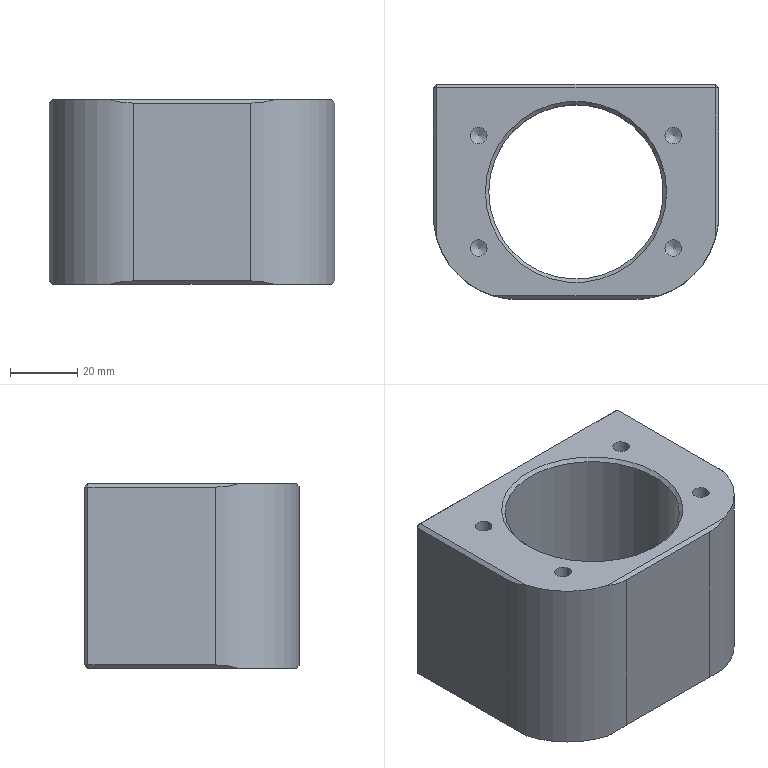Part | NX | 1 solid | 49 faces | box 85 x 64 x 55 mm | volume 163326 mm3 | plane 20 | cylinder 15 | cone 14 | commonest cylinder face diameters 2.5 x4 5 x4 6.8 x4 50 x2 52 x1
STEP:
#1=CARTESIAN_POINT('',(42.5,31.,54.));
#2=VERTEX_POINT('',#1);
#3=CARTESIAN_POINT('',(42.5,-7.,54.));
#4=VERTEX_POINT('',#3);
#5=CARTESIAN_POINT('',(42.5,-32.,54.));
#6=DIRECTION('',(0.,-1.,0.));
#7=VECTOR('',#6,1000.);
#8=LINE('',#5,#7);
#9=EDGE_CURVE('',#2,#4,#8,.T.);
#10=ORIENTED_EDGE('',*,*,#9,.T.);
#11=CARTESIAN_POINT('',(42.5,-7.,1.));
#12=VERTEX_POINT('',#11);
#13=CARTESIAN_POINT('',(42.5,-7.,55.));
#14=DIRECTION('',(0.,0.,-1.));
#15=VECTOR('',#14,1000.);
#16=LINE('',#13,#15);
#17=EDGE_CURVE('',#4,#12,#16,.T.);
#18=ORIENTED_EDGE('',*,*,#17,.T.);
#19=CARTESIAN_POINT('',(42.5,31.,1.));
#20=VERTEX_POINT('',#19);
#21=CARTESIAN_POINT('',(42.5,32.,1.));
#22=DIRECTION('',(0.,1.,0.));
#23=VECTOR('',#22,1000.);
#24=LINE('',#21,#23);
#25=EDGE_CURVE('',#12,#20,#24,.T.);
#26=ORIENTED_EDGE('',*,*,#25,.T.);
#27=CARTESIAN_POINT('',(42.5,31.,55.));
#28=DIRECTION('',(0.,0.,1.));
#29=VECTOR('',#28,1000.);
#30=LINE('',#27,#29);
#31=EDGE_CURVE('',#20,#2,#30,.T.);
#32=ORIENTED_EDGE('',*,*,#31,.T.);
#33=EDGE_LOOP('',(#10,#18,#26,#32));
#34=FACE_BOUND('',#33,.T.);
#35=CARTESIAN_POINT('',(42.5,-32.,55.));
#36=DIRECTION('',(-1.,0.,0.));
#37=DIRECTION('',(0.,0.,1.));
#38=AXIS2_PLACEMENT_3D('',#35,#36,#37);
#39=PLANE('',#38);
#40=ADVANCED_FACE('',(#34),#39,.F.);
#41=CARTESIAN_POINT('',(41.5,32.,54.));
#42=VERTEX_POINT('',#41);
#43=CARTESIAN_POINT('',(41.5,32.,1.));
#44=VERTEX_POINT('',#43);
#45=CARTESIAN_POINT('',(41.5,32.,55.));
#46=DIRECTION('',(0.,0.,-1.));
#47=VECTOR('',#46,1000.);
#48=LINE('',#45,#47);
#49=EDGE_CURVE('',#42,#44,#48,.T.);
#50=ORIENTED_EDGE('',*,*,#49,.T.);
#51=CARTESIAN_POINT('',(-41.5,32.,1.));
#52=VERTEX_POINT('',#51);
#53=CARTESIAN_POINT('',(-42.5,32.,1.));
#54=DIRECTION('',(-1.,0.,0.));
#55=VECTOR('',#54,1000.);
#56=LINE('',#53,#55);
#57=EDGE_CURVE('',#44,#52,#56,.T.);
#58=ORIENTED_EDGE('',*,*,#57,.T.);
#59=CARTESIAN_POINT('',(-41.5,32.,54.));
#60=VERTEX_POINT('',#59);
#61=CARTESIAN_POINT('',(-41.5,32.,55.));
#62=DIRECTION('',(0.,0.,1.));
#63=VECTOR('',#62,1000.);
#64=LINE('',#61,#63);
#65=EDGE_CURVE('',#52,#60,#64,.T.);
#66=ORIENTED_EDGE('',*,*,#65,.T.);
#67=CARTESIAN_POINT('',(-42.5,32.,54.));
#68=DIRECTION('',(1.,0.,0.));
#69=VECTOR('',#68,1000.);
#70=LINE('',#67,#69);
#71=EDGE_CURVE('',#60,#42,#70,.T.);
#72=ORIENTED_EDGE('',*,*,#71,.T.);
#73=EDGE_LOOP('',(#50,#58,#66,#72));
#74=FACE_BOUND('',#73,.T.);
#75=CARTESIAN_POINT('',(35.,32.,13.4));
#76=VERTEX_POINT('',#75);
#77=CARTESIAN_POINT('',(35.,32.,10.));
#78=DIRECTION('',(0.,1.,0.));
#79=DIRECTION('',(0.,0.,1.));
#80=AXIS2_PLACEMENT_3D('',#77,#78,#79);
#81=CIRCLE('',#80,3.4);
#82=EDGE_CURVE('',#76,#76,#81,.T.);
#83=ORIENTED_EDGE('',*,*,#82,.F.);
#84=EDGE_LOOP('',(#83));
#85=FACE_BOUND('',#84,.T.);
#86=CARTESIAN_POINT('',(-35.,32.,13.4));
#87=VERTEX_POINT('',#86);
#88=CARTESIAN_POINT('',(-35.,32.,10.));
#89=DIRECTION('',(0.,1.,0.));
#90=DIRECTION('',(0.,0.,1.));
#91=AXIS2_PLACEMENT_3D('',#88,#89,#90);
#92=CIRCLE('',#91,3.4);
#93=EDGE_CURVE('',#87,#87,#92,.T.);
#94=ORIENTED_EDGE('',*,*,#93,.F.);
#95=EDGE_LOOP('',(#94));
#96=FACE_BOUND('',#95,.T.);
#97=CARTESIAN_POINT('',(35.,32.,48.4));
#98=VERTEX_POINT('',#97);
#99=CARTESIAN_POINT('',(35.,32.,45.));
#100=DIRECTION('',(0.,1.,0.));
#101=DIRECTION('',(0.,0.,1.));
#102=AXIS2_PLACEMENT_3D('',#99,#100,#101);
#103=CIRCLE('',#102,3.4);
#104=EDGE_CURVE('',#98,#98,#103,.T.);
#105=ORIENTED_EDGE('',*,*,#104,.F.);
#106=EDGE_LOOP('',(#105));
#107=FACE_BOUND('',#106,.T.);
#108=CARTESIAN_POINT('',(-35.,32.,48.4));
#109=VERTEX_POINT('',#108);
#110=CARTESIAN_POINT('',(-35.,32.,45.));
#111=DIRECTION('',(0.,1.,0.));
#112=DIRECTION('',(0.,0.,1.));
#113=AXIS2_PLACEMENT_3D('',#110,#111,#112);
#114=CIRCLE('',#113,3.4);
#115=EDGE_CURVE('',#109,#109,#114,.T.);
#116=ORIENTED_EDGE('',*,*,#115,.F.);
#117=EDGE_LOOP('',(#116));
#118=FACE_BOUND('',#117,.T.);
#119=CARTESIAN_POINT('',(-42.5,32.,55.));
#120=DIRECTION('',(0.,-1.,0.));
#121=DIRECTION('',(0.,0.,-1.));
#122=AXIS2_PLACEMENT_3D('',#119,#120,#121);
#123=PLANE('',#122);
#124=ADVANCED_FACE('',(#74,#85,#96,#107,#118),#123,.F.);
#125=CARTESIAN_POINT('',(-42.5,31.,1.));
#126=VERTEX_POINT('',#125);
#127=CARTESIAN_POINT('',(-42.5,-7.,1.));
#128=VERTEX_POINT('',#127);
#129=CARTESIAN_POINT('',(-42.5,-32.,1.));
#130=DIRECTION('',(0.,-1.,0.));
#131=VECTOR('',#130,1000.);
#132=LINE('',#129,#131);
#133=EDGE_CURVE('',#126,#128,#132,.T.);
#134=ORIENTED_EDGE('',*,*,#133,.T.);
#135=CARTESIAN_POINT('',(-42.5,-7.,54.));
#136=VERTEX_POINT('',#135);
#137=CARTESIAN_POINT('',(-42.5,-7.,55.));
#138=DIRECTION('',(0.,0.,-1.));
#139=VECTOR('',#138,1000.);
#140=LINE('',#137,#139);
#141=EDGE_CURVE('',#128,#136,#140,.F.);
#142=ORIENTED_EDGE('',*,*,#141,.T.);
#143=CARTESIAN_POINT('',(-42.5,31.,54.));
#144=VERTEX_POINT('',#143);
#145=CARTESIAN_POINT('',(-42.5,-32.,54.));
#146=DIRECTION('',(0.,1.,0.));
#147=VECTOR('',#146,1000.);
#148=LINE('',#145,#147);
#149=EDGE_CURVE('',#136,#144,#148,.T.);
#150=ORIENTED_EDGE('',*,*,#149,.T.);
#151=CARTESIAN_POINT('',(-42.5,31.,55.));
#152=DIRECTION('',(0.,0.,-1.));
#153=VECTOR('',#152,1000.);
#154=LINE('',#151,#153);
#155=EDGE_CURVE('',#144,#126,#154,.T.);
#156=ORIENTED_EDGE('',*,*,#155,.T.);
#157=EDGE_LOOP('',(#134,#142,#150,#156));
#158=FACE_BOUND('',#157,.T.);
#159=CARTESIAN_POINT('',(-42.5,-32.,55.));
#160=DIRECTION('',(1.,0.,0.));
#161=DIRECTION('',(0.,0.,-1.));
#162=AXIS2_PLACEMENT_3D('',#159,#160,#161);
#163=PLANE('',#162);
#164=ADVANCED_FACE('',(#158),#163,.F.);
#165=CARTESIAN_POINT('',(17.5,-32.,54.));
#166=VERTEX_POINT('',#165);
#167=CARTESIAN_POINT('',(-17.5,-32.,54.));
#168=VERTEX_POINT('',#167);
#169=CARTESIAN_POINT('',(-42.5,-32.,54.));
#170=DIRECTION('',(-1.,0.,0.));
#171=VECTOR('',#170,1000.);
#172=LINE('',#169,#171);
#173=EDGE_CURVE('',#166,#168,#172,.T.);
#174=ORIENTED_EDGE('',*,*,#173,.T.);
#175=CARTESIAN_POINT('',(-17.5,-32.,1.));
#176=VERTEX_POINT('',#175);
#177=CARTESIAN_POINT('',(-17.5,-32.,55.));
#178=DIRECTION('',(0.,0.,-1.));
#179=VECTOR('',#178,1000.);
#180=LINE('',#177,#179);
#181=EDGE_CURVE('',#168,#176,#180,.T.);
#182=ORIENTED_EDGE('',*,*,#181,.T.);
#183=CARTESIAN_POINT('',(17.5,-32.,1.));
#184=VERTEX_POINT('',#183);
#185=CARTESIAN_POINT('',(42.5,-32.,1.));
#186=DIRECTION('',(1.,0.,0.));
#187=VECTOR('',#186,1000.);
#188=LINE('',#185,#187);
#189=EDGE_CURVE('',#176,#184,#188,.T.);
#190=ORIENTED_EDGE('',*,*,#189,.T.);
#191=CARTESIAN_POINT('',(17.5,-32.,55.));
#192=DIRECTION('',(0.,0.,-1.));
#193=VECTOR('',#192,1000.);
#194=LINE('',#191,#193);
#195=EDGE_CURVE('',#184,#166,#194,.F.);
#196=ORIENTED_EDGE('',*,*,#195,.T.);
#197=EDGE_LOOP('',(#174,#182,#190,#196));
#198=FACE_BOUND('',#197,.T.);
#199=CARTESIAN_POINT('',(-42.5,-32.,55.));
#200=DIRECTION('',(0.,1.,0.));
#201=DIRECTION('',(0.,0.,1.));
#202=AXIS2_PLACEMENT_3D('',#199,#200,#201);
#203=PLANE('',#202);
#204=ADVANCED_FACE('',(#198),#203,.F.);
#205=CARTESIAN_POINT('',(-27.,0.,55.));
#206=VERTEX_POINT('',#205);
#207=CARTESIAN_POINT('',(0.,0.,55.));
#208=DIRECTION('',(0.,0.,-1.));
#209=DIRECTION('',(-1.,0.,0.));
#210=AXIS2_PLACEMENT_3D('',#207,#208,#209);
#211=CIRCLE('',#210,27.);
#212=EDGE_CURVE('',#206,#206,#211,.T.);
#213=ORIENTED_EDGE('',*,*,#212,.T.);
#214=EDGE_LOOP('',(#213));
#215=FACE_BOUND('',#214,.T.);
#216=CARTESIAN_POINT('',(-41.5,31.,55.));
#217=VERTEX_POINT('',#216);
#218=CARTESIAN_POINT('',(-41.5,-14.,55.));
#219=VERTEX_POINT('',#218);
#220=CARTESIAN_POINT('',(-41.5,32.,55.));
#221=DIRECTION('',(0.,-1.,0.));
#222=VECTOR('',#221,1000.);
#223=LINE('',#220,#222);
#224=EDGE_CURVE('',#217,#219,#223,.T.);
#225=ORIENTED_EDGE('',*,*,#224,.T.);
#226=CARTESIAN_POINT('',(-24.5,-31.,55.));
#227=VERTEX_POINT('',#226);
#228=CARTESIAN_POINT('',(-17.5,-7.,55.));
#229=DIRECTION('',(0.,0.,-1.));
#230=DIRECTION('',(-1.,0.,0.));
#231=AXIS2_PLACEMENT_3D('',#228,#229,#230);
#232=CIRCLE('',#231,25.);
#233=EDGE_CURVE('',#219,#227,#232,.F.);
#234=ORIENTED_EDGE('',*,*,#233,.T.);
#235=CARTESIAN_POINT('',(24.5,-31.,55.));
#236=VERTEX_POINT('',#235);
#237=CARTESIAN_POINT('',(42.5,-31.,55.));
#238=DIRECTION('',(1.,0.,0.));
#239=VECTOR('',#238,1000.);
#240=LINE('',#237,#239);
#241=EDGE_CURVE('',#227,#236,#240,.T.);
#242=ORIENTED_EDGE('',*,*,#241,.T.);
#243=CARTESIAN_POINT('',(41.5,-14.,55.));
#244=VERTEX_POINT('',#243);
#245=CARTESIAN_POINT('',(17.5,-7.,55.));
#246=DIRECTION('',(0.,0.,-1.));
#247=DIRECTION('',(-1.,0.,0.));
#248=AXIS2_PLACEMENT_3D('',#245,#246,#247);
#249=CIRCLE('',#248,25.);
#250=EDGE_CURVE('',#236,#244,#249,.F.);
#251=ORIENTED_EDGE('',*,*,#250,.T.);
#252=CARTESIAN_POINT('',(41.5,31.,55.));
#253=VERTEX_POINT('',#252);
#254=CARTESIAN_POINT('',(41.5,32.,55.));
#255=DIRECTION('',(0.,1.,0.));
#256=VECTOR('',#255,1000.);
#257=LINE('',#254,#256);
#258=EDGE_CURVE('',#244,#253,#257,.T.);
#259=ORIENTED_EDGE('',*,*,#258,.T.);
#260=CARTESIAN_POINT('',(42.5,31.,55.));
#261=DIRECTION('',(-1.,0.,0.));
#262=VECTOR('',#261,1000.);
#263=LINE('',#260,#262);
#264=EDGE_CURVE('',#253,#217,#263,.T.);
#265=ORIENTED_EDGE('',*,*,#264,.T.);
#266=EDGE_LOOP('',(#225,#234,#242,#251,#259,#265));
#267=FACE_BOUND('',#266,.T.);
#268=CARTESIAN_POINT('',(31.512,16.75,55.));
#269=VERTEX_POINT('',#268);
#270=CARTESIAN_POINT('',(29.012,16.75,55.));
#271=DIRECTION('',(0.,0.,1.));
#272=DIRECTION('',(1.,0.,0.));
#273=AXIS2_PLACEMENT_3D('',#270,#271,#272);
#274=CIRCLE('',#273,2.5);
#275=EDGE_CURVE('',#269,#269,#274,.T.);
#276=ORIENTED_EDGE('',*,*,#275,.F.);
#277=EDGE_LOOP('',(#276));
#278=FACE_BOUND('',#277,.T.);
#279=CARTESIAN_POINT('',(-26.512,16.75,55.));
#280=VERTEX_POINT('',#279);
#281=CARTESIAN_POINT('',(-29.012,16.75,55.));
#282=DIRECTION('',(0.,0.,1.));
#283=DIRECTION('',(1.,0.,0.));
#284=AXIS2_PLACEMENT_3D('',#281,#282,#283);
#285=CIRCLE('',#284,2.5);
#286=EDGE_CURVE('',#280,#280,#285,.T.);
#287=ORIENTED_EDGE('',*,*,#286,.F.);
#288=EDGE_LOOP('',(#287));
#289=FACE_BOUND('',#288,.T.);
#290=CARTESIAN_POINT('',(-26.512,-16.75,55.));
#291=VERTEX_POINT('',#290);
#292=CARTESIAN_POINT('',(-29.012,-16.75,55.));
#293=DIRECTION('',(0.,0.,1.));
#294=DIRECTION('',(1.,0.,0.));
#295=AXIS2_PLACEMENT_3D('',#292,#293,#294);
#296=CIRCLE('',#295,2.5);
#297=EDGE_CURVE('',#291,#291,#296,.T.);
#298=ORIENTED_EDGE('',*,*,#297,.F.);
#299=EDGE_LOOP('',(#298));
#300=FACE_BOUND('',#299,.T.);
#301=CARTESIAN_POINT('',(31.512,-16.75,55.));
#302=VERTEX_POINT('',#301);
#303=CARTESIAN_POINT('',(29.012,-16.75,55.));
#304=DIRECTION('',(0.,0.,1.));
#305=DIRECTION('',(1.,0.,0.));
#306=AXIS2_PLACEMENT_3D('',#303,#304,#305);
#307=CIRCLE('',#306,2.5);
#308=EDGE_CURVE('',#302,#302,#307,.T.);
#309=ORIENTED_EDGE('',*,*,#308,.F.);
#310=EDGE_LOOP('',(#309));
#311=FACE_BOUND('',#310,.T.);
#312=CARTESIAN_POINT('',(42.5,32.,55.));
#313=DIRECTION('',(0.,0.,-1.));
#314=DIRECTION('',(-1.,0.,0.));
#315=AXIS2_PLACEMENT_3D('',#312,#313,#314);
#316=PLANE('',#315);
#317=ADVANCED_FACE('',(#215,#267,#278,#289,#300,#311),#316,.F.);
#318=CARTESIAN_POINT('',(28.75,22.,0.));
#319=VERTEX_POINT('',#318);
#320=CARTESIAN_POINT('',(30.,22.,0.));
#321=DIRECTION('',(0.,0.,-1.));
#322=DIRECTION('',(-1.,0.,0.));
#323=AXIS2_PLACEMENT_3D('',#320,#321,#322);
#324=CIRCLE('',#323,1.25);
#325=EDGE_CURVE('',#319,#319,#324,.T.);
#326=ORIENTED_EDGE('',*,*,#325,.F.);
#327=EDGE_LOOP('',(#326));
#328=FACE_BOUND('',#327,.T.);
#329=CARTESIAN_POINT('',(-31.25,22.,0.));
#330=VERTEX_POINT('',#329);
#331=CARTESIAN_POINT('',(-30.,22.,0.));
#332=DIRECTION('',(0.,0.,-1.));
#333=DIRECTION('',(-1.,0.,0.));
#334=AXIS2_PLACEMENT_3D('',#331,#332,#333);
#335=CIRCLE('',#334,1.25);
#336=EDGE_CURVE('',#330,#330,#335,.T.);
#337=ORIENTED_EDGE('',*,*,#336,.F.);
#338=EDGE_LOOP('',(#337));
#339=FACE_BOUND('',#338,.T.);
#340=CARTESIAN_POINT('',(-31.25,-13.,0.));
#341=VERTEX_POINT('',#340);
#342=CARTESIAN_POINT('',(-30.,-13.,0.));
#343=DIRECTION('',(0.,0.,-1.));
#344=DIRECTION('',(-1.,0.,0.));
#345=AXIS2_PLACEMENT_3D('',#342,#343,#344);
#346=CIRCLE('',#345,1.25);
#347=EDGE_CURVE('',#341,#341,#346,.T.);
#348=ORIENTED_EDGE('',*,*,#347,.F.);
#349=EDGE_LOOP('',(#348));
#350=FACE_BOUND('',#349,.T.);
#351=CARTESIAN_POINT('',(28.75,-13.,0.));
#352=VERTEX_POINT('',#351);
#353=CARTESIAN_POINT('',(30.,-13.,0.));
#354=DIRECTION('',(0.,0.,-1.));
#355=DIRECTION('',(-1.,0.,0.));
#356=AXIS2_PLACEMENT_3D('',#353,#354,#355);
#357=CIRCLE('',#356,1.25);
#358=EDGE_CURVE('',#352,#352,#357,.T.);
#359=ORIENTED_EDGE('',*,*,#358,.F.);
#360=EDGE_LOOP('',(#359));
#361=FACE_BOUND('',#360,.T.);
#362=CARTESIAN_POINT('',(-27.,0.,0.));
#363=VERTEX_POINT('',#362);
#364=CARTESIAN_POINT('',(0.,0.,0.));
#365=DIRECTION('',(0.,0.,-1.));
#366=DIRECTION('',(-1.,0.,0.));
#367=AXIS2_PLACEMENT_3D('',#364,#365,#366);
#368=CIRCLE('',#367,27.);
#369=EDGE_CURVE('',#363,#363,#368,.F.);
#370=ORIENTED_EDGE('',*,*,#369,.T.);
#371=EDGE_LOOP('',(#370));
#372=FACE_BOUND('',#371,.T.);
#373=CARTESIAN_POINT('',(24.5,-31.,0.));
#374=VERTEX_POINT('',#373);
#375=CARTESIAN_POINT('',(-24.5,-31.,0.));
#376=VERTEX_POINT('',#375);
#377=CARTESIAN_POINT('',(-42.5,-31.,0.));
#378=DIRECTION('',(-1.,0.,0.));
#379=VECTOR('',#378,1000.);
#380=LINE('',#377,#379);
#381=EDGE_CURVE('',#374,#376,#380,.T.);
#382=ORIENTED_EDGE('',*,*,#381,.T.);
#383=CARTESIAN_POINT('',(-41.5,-14.,0.));
#384=VERTEX_POINT('',#383);
#385=CARTESIAN_POINT('',(-17.5,-7.,0.));
#386=DIRECTION('',(0.,0.,-1.));
#387=DIRECTION('',(-1.,0.,0.));
#388=AXIS2_PLACEMENT_3D('',#385,#386,#387);
#389=CIRCLE('',#388,25.);
#390=EDGE_CURVE('',#376,#384,#389,.T.);
#391=ORIENTED_EDGE('',*,*,#390,.T.);
#392=CARTESIAN_POINT('',(-41.5,31.,0.));
#393=VERTEX_POINT('',#392);
#394=CARTESIAN_POINT('',(-41.5,32.,0.));
#395=DIRECTION('',(0.,1.,0.));
#396=VECTOR('',#395,1000.);
#397=LINE('',#394,#396);
#398=EDGE_CURVE('',#384,#393,#397,.T.);
#399=ORIENTED_EDGE('',*,*,#398,.T.);
#400=CARTESIAN_POINT('',(41.5,31.,0.));
#401=VERTEX_POINT('',#400);
#402=CARTESIAN_POINT('',(42.5,31.,0.));
#403=DIRECTION('',(1.,0.,0.));
#404=VECTOR('',#403,1000.);
#405=LINE('',#402,#404);
#406=EDGE_CURVE('',#393,#401,#405,.T.);
#407=ORIENTED_EDGE('',*,*,#406,.T.);
#408=CARTESIAN_POINT('',(41.5,-14.,0.));
#409=VERTEX_POINT('',#408);
#410=CARTESIAN_POINT('',(41.5,-32.,0.));
#411=DIRECTION('',(0.,-1.,0.));
#412=VECTOR('',#411,1000.);
#413=LINE('',#410,#412);
#414=EDGE_CURVE('',#401,#409,#413,.T.);
#415=ORIENTED_EDGE('',*,*,#414,.T.);
#416=CARTESIAN_POINT('',(17.5,-7.,0.));
#417=DIRECTION('',(0.,0.,-1.));
#418=DIRECTION('',(-1.,0.,0.));
#419=AXIS2_PLACEMENT_3D('',#416,#417,#418);
#420=CIRCLE('',#419,25.);
#421=EDGE_CURVE('',#409,#374,#420,.T.);
#422=ORIENTED_EDGE('',*,*,#421,.T.);
#423=EDGE_LOOP('',(#382,#391,#399,#407,#415,#422));
#424=FACE_BOUND('',#423,.T.);
#425=CARTESIAN_POINT('',(42.5,32.,0.));
#426=DIRECTION('',(0.,0.,-1.));
#427=DIRECTION('',(-1.,0.,0.));
#428=AXIS2_PLACEMENT_3D('',#425,#426,#427);
#429=PLANE('',#428);
#430=ADVANCED_FACE('',(#328,#339,#350,#361,#372,#424),#429,.T.);
#431=CARTESIAN_POINT('',(-26.,0.,54.));
#432=VERTEX_POINT('',#431);
#433=CARTESIAN_POINT('',(0.,0.,54.));
#434=DIRECTION('',(0.,0.,-1.));
#435=DIRECTION('',(-1.,0.,0.));
#436=AXIS2_PLACEMENT_3D('',#433,#434,#435);
#437=CIRCLE('',#436,26.);
#438=EDGE_CURVE('',#432,#432,#437,.F.);
#439=ORIENTED_EDGE('',*,*,#438,.T.);
#440=EDGE_LOOP('',(#439));
#441=FACE_BOUND('',#440,.T.);
#442=CARTESIAN_POINT('',(-26.,0.,1.));
#443=VERTEX_POINT('',#442);
#444=CARTESIAN_POINT('',(0.,0.,1.));
#445=DIRECTION('',(0.,0.,-1.));
#446=DIRECTION('',(-1.,0.,0.));
#447=AXIS2_PLACEMENT_3D('',#444,#445,#446);
#448=CIRCLE('',#447,26.);
#449=EDGE_CURVE('',#443,#443,#448,.T.);
#450=ORIENTED_EDGE('',*,*,#449,.T.);
#451=EDGE_LOOP('',(#450));
#452=FACE_BOUND('',#451,.T.);
#453=CARTESIAN_POINT('',(0.,0.,0.));
#454=DIRECTION('',(0.,0.,1.));
#455=DIRECTION('',(1.,0.,0.));
#456=AXIS2_PLACEMENT_3D('',#453,#454,#455);
#457=CYLINDRICAL_SURFACE('',#456,26.);
#458=ADVANCED_FACE('',(#441,#452),#457,.F.);
#459=CARTESIAN_POINT('',(-35.,13.457,45.));
#460=VERTEX_POINT('',#459);
#461=VERTEX_LOOP('',#460);
#462=FACE_BOUND('',#461,.T.);
#463=CARTESIAN_POINT('',(-35.,15.5,48.4));
#464=VERTEX_POINT('',#463);
#465=CARTESIAN_POINT('',(-35.,15.5,45.));
#466=DIRECTION('',(0.,1.,0.));
#467=DIRECTION('',(0.,0.,1.));
#468=AXIS2_PLACEMENT_3D('',#465,#466,#467);
#469=CIRCLE('',#468,3.4);
#470=EDGE_CURVE('',#464,#464,#469,.T.);
#471=ORIENTED_EDGE('',*,*,#470,.T.);
#472=EDGE_LOOP('',(#471));
#473=FACE_BOUND('',#472,.T.);
#474=CARTESIAN_POINT('',(-35.,15.5,45.));
#475=DIRECTION('',(0.,1.,0.));
#476=DIRECTION('',(0.,0.,1.));
#477=AXIS2_PLACEMENT_3D('',#474,#475,#476);
#478=CONICAL_SURFACE('',#477,3.4,1.03);
#479=ADVANCED_FACE('',(#462,#473),#478,.F.);
#480=ORIENTED_EDGE('',*,*,#470,.F.);
#481=EDGE_LOOP('',(#480));
#482=FACE_BOUND('',#481,.T.);
#483=ORIENTED_EDGE('',*,*,#115,.T.);
#484=EDGE_LOOP('',(#483));
#485=FACE_BOUND('',#484,.T.);
#486=CARTESIAN_POINT('',(-35.,32.,45.));
#487=DIRECTION('',(0.,1.,0.));
#488=DIRECTION('',(0.,0.,1.));
#489=AXIS2_PLACEMENT_3D('',#486,#487,#488);
#490=CYLINDRICAL_SURFACE('',#489,3.4);
#491=ADVANCED_FACE('',(#482,#485),#490,.F.);
#492=CARTESIAN_POINT('',(35.,13.457,45.));
#493=VERTEX_POINT('',#492);
#494=VERTEX_LOOP('',#493);
#495=FACE_BOUND('',#494,.T.);
#496=CARTESIAN_POINT('',(35.,15.5,48.4));
#497=VERTEX_POINT('',#496);
#498=CARTESIAN_POINT('',(35.,15.5,45.));
#499=DIRECTION('',(0.,1.,0.));
#500=DIRECTION('',(0.,0.,1.));
#501=AXIS2_PLACEMENT_3D('',#498,#499,#500);
#502=CIRCLE('',#501,3.4);
#503=EDGE_CURVE('',#497,#497,#502,.T.);
#504=ORIENTED_EDGE('',*,*,#503,.T.);
#505=EDGE_LOOP('',(#504));
#506=FACE_BOUND('',#505,.T.);
#507=CARTESIAN_POINT('',(35.,15.5,45.));
#508=DIRECTION('',(0.,1.,0.));
#509=DIRECTION('',(0.,0.,1.));
#510=AXIS2_PLACEMENT_3D('',#507,#508,#509);
#511=CONICAL_SURFACE('',#510,3.4,1.03);
#512=ADVANCED_FACE('',(#495,#506),#511,.F.);
#513=ORIENTED_EDGE('',*,*,#503,.F.);
#514=EDGE_LOOP('',(#513));
#515=FACE_BOUND('',#514,.T.);
#516=ORIENTED_EDGE('',*,*,#104,.T.);
#517=EDGE_LOOP('',(#516));
#518=FACE_BOUND('',#517,.T.);
#519=CARTESIAN_POINT('',(35.,32.,45.));
#520=DIRECTION('',(0.,1.,0.));
#521=DIRECTION('',(0.,0.,1.));
#522=AXIS2_PLACEMENT_3D('',#519,#520,#521);
#523=CYLINDRICAL_SURFACE('',#522,3.4);
#524=ADVANCED_FACE('',(#515,#518),#523,.F.);
#525=CARTESIAN_POINT('',(-35.,13.457,10.));
#526=VERTEX_POINT('',#525);
#527=VERTEX_LOOP('',#526);
#528=FACE_BOUND('',#527,.T.);
#529=CARTESIAN_POINT('',(-35.,15.5,13.4));
#530=VERTEX_POINT('',#529);
#531=CARTESIAN_POINT('',(-35.,15.5,10.));
#532=DIRECTION('',(0.,1.,0.));
#533=DIRECTION('',(0.,0.,1.));
#534=AXIS2_PLACEMENT_3D('',#531,#532,#533);
#535=CIRCLE('',#534,3.4);
#536=EDGE_CURVE('',#530,#530,#535,.T.);
#537=ORIENTED_EDGE('',*,*,#536,.T.);
#538=EDGE_LOOP('',(#537));
#539=FACE_BOUND('',#538,.T.);
#540=CARTESIAN_POINT('',(-35.,15.5,10.));
#541=DIRECTION('',(0.,1.,0.));
#542=DIRECTION('',(0.,0.,1.));
#543=AXIS2_PLACEMENT_3D('',#540,#541,#542);
#544=CONICAL_SURFACE('',#543,3.4,1.03);
#545=ADVANCED_FACE('',(#528,#539),#544,.F.);
#546=ORIENTED_EDGE('',*,*,#536,.F.);
#547=EDGE_LOOP('',(#546));
#548=FACE_BOUND('',#547,.T.);
#549=ORIENTED_EDGE('',*,*,#93,.T.);
#550=EDGE_LOOP('',(#549));
#551=FACE_BOUND('',#550,.T.);
#552=CARTESIAN_POINT('',(-35.,32.,10.));
#553=DIRECTION('',(0.,1.,0.));
#554=DIRECTION('',(0.,0.,1.));
#555=AXIS2_PLACEMENT_3D('',#552,#553,#554);
#556=CYLINDRICAL_SURFACE('',#555,3.4);
#557=ADVANCED_FACE('',(#548,#551),#556,.F.);
#558=CARTESIAN_POINT('',(35.,13.457,10.));
#559=VERTEX_POINT('',#558);
#560=VERTEX_LOOP('',#559);
#561=FACE_BOUND('',#560,.T.);
#562=CARTESIAN_POINT('',(35.,15.5,13.4));
#563=VERTEX_POINT('',#562);
#564=CARTESIAN_POINT('',(35.,15.5,10.));
#565=DIRECTION('',(0.,1.,0.));
#566=DIRECTION('',(0.,0.,1.));
#567=AXIS2_PLACEMENT_3D('',#564,#565,#566);
#568=CIRCLE('',#567,3.4);
#569=EDGE_CURVE('',#563,#563,#568,.T.);
#570=ORIENTED_EDGE('',*,*,#569,.T.);
#571=EDGE_LOOP('',(#570));
#572=FACE_BOUND('',#571,.T.);
#573=CARTESIAN_POINT('',(35.,15.5,10.));
#574=DIRECTION('',(0.,1.,0.));
#575=DIRECTION('',(0.,0.,1.));
#576=AXIS2_PLACEMENT_3D('',#573,#574,#575);
#577=CONICAL_SURFACE('',#576,3.4,1.03);
#578=ADVANCED_FACE('',(#561,#572),#577,.F.);
#579=ORIENTED_EDGE('',*,*,#569,.F.);
#580=EDGE_LOOP('',(#579));
#581=FACE_BOUND('',#580,.T.);
#582=ORIENTED_EDGE('',*,*,#82,.T.);
#583=EDGE_LOOP('',(#582));
#584=FACE_BOUND('',#583,.T.);
#585=CARTESIAN_POINT('',(35.,32.,10.));
#586=DIRECTION('',(0.,1.,0.));
#587=DIRECTION('',(0.,0.,1.));
#588=AXIS2_PLACEMENT_3D('',#585,#586,#587);
#589=CYLINDRICAL_SURFACE('',#588,3.4);
#590=ADVANCED_FACE('',(#581,#584),#589,.F.);
#591=CARTESIAN_POINT('',(29.012,-16.75,38.498));
#592=VERTEX_POINT('',#591);
#593=VERTEX_LOOP('',#592);
#594=FACE_BOUND('',#593,.T.);
#595=CARTESIAN_POINT('',(31.512,-16.75,40.));
#596=VERTEX_POINT('',#595);
#597=CARTESIAN_POINT('',(29.012,-16.75,40.));
#598=DIRECTION('',(0.,0.,1.));
#599=DIRECTION('',(1.,0.,0.));
#600=AXIS2_PLACEMENT_3D('',#597,#598,#599);
#601=CIRCLE('',#600,2.5);
#602=EDGE_CURVE('',#596,#596,#601,.T.);
#603=ORIENTED_EDGE('',*,*,#602,.T.);
#604=EDGE_LOOP('',(#603));
#605=FACE_BOUND('',#604,.T.);
#606=CARTESIAN_POINT('',(29.012,-16.75,40.));
#607=DIRECTION('',(0.,0.,1.));
#608=DIRECTION('',(1.,0.,0.));
#609=AXIS2_PLACEMENT_3D('',#606,#607,#608);
#610=CONICAL_SURFACE('',#609,2.5,1.03);
#611=ADVANCED_FACE('',(#594,#605),#610,.F.);
#612=ORIENTED_EDGE('',*,*,#602,.F.);
#613=EDGE_LOOP('',(#612));
#614=FACE_BOUND('',#613,.T.);
#615=ORIENTED_EDGE('',*,*,#308,.T.);
#616=EDGE_LOOP('',(#615));
#617=FACE_BOUND('',#616,.T.);
#618=CARTESIAN_POINT('',(29.012,-16.75,55.));
#619=DIRECTION('',(0.,0.,1.));
#620=DIRECTION('',(1.,0.,0.));
#621=AXIS2_PLACEMENT_3D('',#618,#619,#620);
#622=CYLINDRICAL_SURFACE('',#621,2.5);
#623=ADVANCED_FACE('',(#614,#617),#622,.F.);
#624=CARTESIAN_POINT('',(-29.012,-16.75,38.498));
#625=VERTEX_POINT('',#624);
#626=VERTEX_LOOP('',#625);
#627=FACE_BOUND('',#626,.T.);
#628=CARTESIAN_POINT('',(-26.512,-16.75,40.));
#629=VERTEX_POINT('',#628);
#630=CARTESIAN_POINT('',(-29.012,-16.75,40.));
#631=DIRECTION('',(0.,0.,1.));
#632=DIRECTION('',(1.,0.,0.));
#633=AXIS2_PLACEMENT_3D('',#630,#631,#632);
#634=CIRCLE('',#633,2.5);
#635=EDGE_CURVE('',#629,#629,#634,.T.);
#636=ORIENTED_EDGE('',*,*,#635,.T.);
#637=EDGE_LOOP('',(#636));
#638=FACE_BOUND('',#637,.T.);
#639=CARTESIAN_POINT('',(-29.012,-16.75,40.));
#640=DIRECTION('',(0.,0.,1.));
#641=DIRECTION('',(1.,0.,0.));
#642=AXIS2_PLACEMENT_3D('',#639,#640,#641);
#643=CONICAL_SURFACE('',#642,2.5,1.03);
#644=ADVANCED_FACE('',(#627,#638),#643,.F.);
#645=ORIENTED_EDGE('',*,*,#635,.F.);
#646=EDGE_LOOP('',(#645));
#647=FACE_BOUND('',#646,.T.);
#648=ORIENTED_EDGE('',*,*,#297,.T.);
#649=EDGE_LOOP('',(#648));
#650=FACE_BOUND('',#649,.T.);
#651=CARTESIAN_POINT('',(-29.012,-16.75,55.));
#652=DIRECTION('',(0.,0.,1.));
#653=DIRECTION('',(1.,0.,0.));
#654=AXIS2_PLACEMENT_3D('',#651,#652,#653);
#655=CYLINDRICAL_SURFACE('',#654,2.5);
#656=ADVANCED_FACE('',(#647,#650),#655,.F.);
#657=CARTESIAN_POINT('',(-29.012,16.75,38.498));
#658=VERTEX_POINT('',#657);
#659=VERTEX_LOOP('',#658);
#660=FACE_BOUND('',#659,.T.);
#661=CARTESIAN_POINT('',(-26.512,16.75,40.));
#662=VERTEX_POINT('',#661);
#663=CARTESIAN_POINT('',(-29.012,16.75,40.));
#664=DIRECTION('',(0.,0.,1.));
#665=DIRECTION('',(1.,0.,0.));
#666=AXIS2_PLACEMENT_3D('',#663,#664,#665);
#667=CIRCLE('',#666,2.5);
#668=EDGE_CURVE('',#662,#662,#667,.T.);
#669=ORIENTED_EDGE('',*,*,#668,.T.);
#670=EDGE_LOOP('',(#669));
#671=FACE_BOUND('',#670,.T.);
#672=CARTESIAN_POINT('',(-29.012,16.75,40.));
#673=DIRECTION('',(0.,0.,1.));
#674=DIRECTION('',(1.,0.,0.));
#675=AXIS2_PLACEMENT_3D('',#672,#673,#674);
#676=CONICAL_SURFACE('',#675,2.5,1.03);
#677=ADVANCED_FACE('',(#660,#671),#676,.F.);
#678=ORIENTED_EDGE('',*,*,#668,.F.);
#679=EDGE_LOOP('',(#678));
#680=FACE_BOUND('',#679,.T.);
#681=ORIENTED_EDGE('',*,*,#286,.T.);
#682=EDGE_LOOP('',(#681));
#683=FACE_BOUND('',#682,.T.);
#684=CARTESIAN_POINT('',(-29.012,16.75,55.));
#685=DIRECTION('',(0.,0.,1.));
#686=DIRECTION('',(1.,0.,0.));
#687=AXIS2_PLACEMENT_3D('',#684,#685,#686);
#688=CYLINDRICAL_SURFACE('',#687,2.5);
#689=ADVANCED_FACE('',(#680,#683),#688,.F.);
#690=CARTESIAN_POINT('',(29.012,16.75,38.498));
#691=VERTEX_POINT('',#690);
#692=VERTEX_LOOP('',#691);
#693=FACE_BOUND('',#692,.T.);
#694=CARTESIAN_POINT('',(31.512,16.75,40.));
#695=VERTEX_POINT('',#694);
#696=CARTESIAN_POINT('',(29.012,16.75,40.));
#697=DIRECTION('',(0.,0.,1.));
#698=DIRECTION('',(1.,0.,0.));
#699=AXIS2_PLACEMENT_3D('',#696,#697,#698);
#700=CIRCLE('',#699,2.5);
#701=EDGE_CURVE('',#695,#695,#700,.T.);
#702=ORIENTED_EDGE('',*,*,#701,.T.);
#703=EDGE_LOOP('',(#702));
#704=FACE_BOUND('',#703,.T.);
#705=CARTESIAN_POINT('',(29.012,16.75,40.));
#706=DIRECTION('',(0.,0.,1.));
#707=DIRECTION('',(1.,0.,0.));
#708=AXIS2_PLACEMENT_3D('',#705,#706,#707);
#709=CONICAL_SURFACE('',#708,2.5,1.03);
#710=ADVANCED_FACE('',(#693,#704),#709,.F.);
#711=ORIENTED_EDGE('',*,*,#701,.F.);
#712=EDGE_LOOP('',(#711));
#713=FACE_BOUND('',#712,.T.);
#714=ORIENTED_EDGE('',*,*,#275,.T.);
#715=EDGE_LOOP('',(#714));
#716=FACE_BOUND('',#715,.T.);
#717=CARTESIAN_POINT('',(29.012,16.75,55.));
#718=DIRECTION('',(0.,0.,1.));
#719=DIRECTION('',(1.,0.,0.));
#720=AXIS2_PLACEMENT_3D('',#717,#718,#719);
#721=CYLINDRICAL_SURFACE('',#720,2.5);
#722=ADVANCED_FACE('',(#713,#716),#721,.F.);
#723=ORIENTED_EDGE('',*,*,#212,.F.);
#724=EDGE_LOOP('',(#723));
#725=FACE_BOUND('',#724,.T.);
#726=ORIENTED_EDGE('',*,*,#438,.F.);
#727=EDGE_LOOP('',(#726));
#728=FACE_BOUND('',#727,.T.);
#729=CARTESIAN_POINT('',(0.,0.,54.));
#730=DIRECTION('',(0.,0.,1.));
#731=DIRECTION('',(1.,0.,0.));
#732=AXIS2_PLACEMENT_3D('',#729,#730,#731);
#733=CONICAL_SURFACE('',#732,26.,0.7854);
#734=ADVANCED_FACE('',(#725,#728),#733,.F.);
#735=ORIENTED_EDGE('',*,*,#449,.F.);
#736=EDGE_LOOP('',(#735));
#737=FACE_BOUND('',#736,.T.);
#738=ORIENTED_EDGE('',*,*,#369,.F.);
#739=EDGE_LOOP('',(#738));
#740=FACE_BOUND('',#739,.T.);
#741=CARTESIAN_POINT('',(0.,0.,0.));
#742=DIRECTION('',(0.,0.,-1.));
#743=DIRECTION('',(-1.,0.,0.));
#744=AXIS2_PLACEMENT_3D('',#741,#742,#743);
#745=CONICAL_SURFACE('',#744,27.,0.7854);
#746=ADVANCED_FACE('',(#737,#740),#745,.F.);
#747=ORIENTED_EDGE('',*,*,#241,.F.);
#748=CARTESIAN_POINT('',(-17.5,-7.,79.));
#749=DIRECTION('',(0.,0.7071,-0.7071));
#750=DIRECTION('',(0.,-0.7071,-0.7071));
#751=AXIS2_PLACEMENT_3D('',#748,#749,#750);
#752=ELLIPSE('',#751,35.355,25.);
#753=EDGE_CURVE('',#227,#168,#752,.F.);
#754=ORIENTED_EDGE('',*,*,#753,.T.);
#755=ORIENTED_EDGE('',*,*,#173,.F.);
#756=CARTESIAN_POINT('',(17.5,-7.,79.));
#757=DIRECTION('',(0.,0.7071,-0.7071));
#758=DIRECTION('',(0.,-0.7071,-0.7071));
#759=AXIS2_PLACEMENT_3D('',#756,#757,#758);
#760=ELLIPSE('',#759,35.355,25.);
#761=EDGE_CURVE('',#166,#236,#760,.F.);
#762=ORIENTED_EDGE('',*,*,#761,.T.);
#763=EDGE_LOOP('',(#747,#754,#755,#762));
#764=FACE_BOUND('',#763,.T.);
#765=CARTESIAN_POINT('',(42.5,-31.,55.));
#766=DIRECTION('',(0.,0.7071,-0.7071));
#767=DIRECTION('',(0.,0.7071,0.7071));
#768=AXIS2_PLACEMENT_3D('',#765,#766,#767);
#769=PLANE('',#768);
#770=ADVANCED_FACE('',(#764),#769,.F.);
#771=ORIENTED_EDGE('',*,*,#149,.F.);
#772=CARTESIAN_POINT('',(-17.5,-7.,79.));
#773=DIRECTION('',(0.7071,0.,-0.7071));
#774=DIRECTION('',(-0.7071,0.,-0.7071));
#775=AXIS2_PLACEMENT_3D('',#772,#773,#774);
#776=ELLIPSE('',#775,35.355,25.);
#777=EDGE_CURVE('',#136,#219,#776,.F.);
#778=ORIENTED_EDGE('',*,*,#777,.T.);
#779=ORIENTED_EDGE('',*,*,#224,.F.);
#780=CARTESIAN_POINT('',(-41.5,31.,55.));
#781=DIRECTION('',(-0.7071,0.,-0.7071));
#782=VECTOR('',#781,1000.);
#783=LINE('',#780,#782);
#784=EDGE_CURVE('',#144,#217,#783,.F.);
#785=ORIENTED_EDGE('',*,*,#784,.F.);
#786=EDGE_LOOP('',(#771,#778,#779,#785));
#787=FACE_BOUND('',#786,.T.);
#788=CARTESIAN_POINT('',(-41.5,32.,55.));
#789=DIRECTION('',(0.7071,0.,-0.7071));
#790=DIRECTION('',(-0.7071,0.,-0.7071));
#791=AXIS2_PLACEMENT_3D('',#788,#789,#790);
#792=PLANE('',#791);
#793=ADVANCED_FACE('',(#787),#792,.F.);
#794=ORIENTED_EDGE('',*,*,#258,.F.);
#795=CARTESIAN_POINT('',(17.5,-7.,79.));
#796=DIRECTION('',(-0.7071,0.,-0.7071));
#797=DIRECTION('',(0.7071,0.,-0.7071));
#798=AXIS2_PLACEMENT_3D('',#795,#796,#797);
#799=ELLIPSE('',#798,35.355,25.);
#800=EDGE_CURVE('',#244,#4,#799,.F.);
#801=ORIENTED_EDGE('',*,*,#800,.T.);
#802=ORIENTED_EDGE('',*,*,#9,.F.);
#803=CARTESIAN_POINT('',(41.5,31.,55.));
#804=DIRECTION('',(-0.7071,0.,0.7071));
#805=VECTOR('',#804,1000.);
#806=LINE('',#803,#805);
#807=EDGE_CURVE('',#253,#2,#806,.F.);
#808=ORIENTED_EDGE('',*,*,#807,.F.);
#809=EDGE_LOOP('',(#794,#801,#802,#808));
#810=FACE_BOUND('',#809,.T.);
#811=CARTESIAN_POINT('',(41.5,32.,55.));
#812=DIRECTION('',(-0.7071,0.,-0.7071));
#813=DIRECTION('',(-0.7071,0.,0.7071));
#814=AXIS2_PLACEMENT_3D('',#811,#812,#813);
#815=PLANE('',#814);
#816=ADVANCED_FACE('',(#810),#815,.F.);
#817=CARTESIAN_POINT('',(-41.5,31.,55.));
#818=DIRECTION('',(0.,-0.7071,0.7071));
#819=VECTOR('',#818,1000.);
#820=LINE('',#817,#819);
#821=EDGE_CURVE('',#217,#60,#820,.F.);
#822=ORIENTED_EDGE('',*,*,#821,.F.);
#823=ORIENTED_EDGE('',*,*,#264,.F.);
#824=CARTESIAN_POINT('',(41.5,31.,55.));
#825=DIRECTION('',(0.,0.7071,-0.7071));
#826=VECTOR('',#825,1000.);
#827=LINE('',#824,#826);
#828=EDGE_CURVE('',#42,#253,#827,.F.);
#829=ORIENTED_EDGE('',*,*,#828,.F.);
#830=ORIENTED_EDGE('',*,*,#71,.F.);
#831=EDGE_LOOP('',(#822,#823,#829,#830));
#832=FACE_BOUND('',#831,.T.);
#833=CARTESIAN_POINT('',(42.5,31.,55.));
#834=DIRECTION('',(0.,-0.7071,-0.7071));
#835=DIRECTION('',(0.,0.7071,-0.7071));
#836=AXIS2_PLACEMENT_3D('',#833,#834,#835);
#837=PLANE('',#836);
#838=ADVANCED_FACE('',(#832),#837,.F.);
#839=ORIENTED_EDGE('',*,*,#784,.T.);
#840=ORIENTED_EDGE('',*,*,#821,.T.);
#841=CARTESIAN_POINT('',(-42.,31.5,54.));
#842=DIRECTION('',(0.7071,0.7071,0.));
#843=VECTOR('',#842,1000.);
#844=LINE('',#841,#843);
#845=EDGE_CURVE('',#144,#60,#844,.T.);
#846=ORIENTED_EDGE('',*,*,#845,.F.);
#847=EDGE_LOOP('',(#839,#840,#846));
#848=FACE_BOUND('',#847,.T.);
#849=CARTESIAN_POINT('',(-41.5,31.,55.));
#850=DIRECTION('',(-0.5774,0.5774,0.5774));
#851=DIRECTION('',(-0.7071,-0.7071,0.));
#852=AXIS2_PLACEMENT_3D('',#849,#850,#851);
#853=PLANE('',#852);
#854=ADVANCED_FACE('',(#848),#853,.T.);
#855=ORIENTED_EDGE('',*,*,#828,.T.);
#856=ORIENTED_EDGE('',*,*,#807,.T.);
#857=CARTESIAN_POINT('',(42.,31.5,54.));
#858=DIRECTION('',(0.7071,-0.7071,0.));
#859=VECTOR('',#858,1000.);
#860=LINE('',#857,#859);
#861=EDGE_CURVE('',#42,#2,#860,.T.);
#862=ORIENTED_EDGE('',*,*,#861,.F.);
#863=EDGE_LOOP('',(#855,#856,#862));
#864=FACE_BOUND('',#863,.T.);
#865=CARTESIAN_POINT('',(41.5,31.,55.));
#866=DIRECTION('',(0.5774,0.5774,0.5774));
#867=DIRECTION('',(-0.7071,0.7071,0.));
#868=AXIS2_PLACEMENT_3D('',#865,#866,#867);
#869=PLANE('',#868);
#870=ADVANCED_FACE('',(#864),#869,.T.);
#871=ORIENTED_EDGE('',*,*,#845,.T.);
#872=ORIENTED_EDGE('',*,*,#65,.F.);
#873=CARTESIAN_POINT('',(-42.,31.5,1.));
#874=DIRECTION('',(-0.7071,-0.7071,0.));
#875=VECTOR('',#874,1000.);
#876=LINE('',#873,#875);
#877=EDGE_CURVE('',#126,#52,#876,.F.);
#878=ORIENTED_EDGE('',*,*,#877,.F.);
#879=ORIENTED_EDGE('',*,*,#155,.F.);
#880=EDGE_LOOP('',(#871,#872,#878,#879));
#881=FACE_BOUND('',#880,.T.);
#882=CARTESIAN_POINT('',(-42.5,31.,55.));
#883=DIRECTION('',(0.7071,-0.7071,0.));
#884=DIRECTION('',(0.7071,0.7071,0.));
#885=AXIS2_PLACEMENT_3D('',#882,#883,#884);
#886=PLANE('',#885);
#887=ADVANCED_FACE('',(#881),#886,.F.);
#888=ORIENTED_EDGE('',*,*,#861,.T.);
#889=ORIENTED_EDGE('',*,*,#31,.F.);
#890=CARTESIAN_POINT('',(42.5,31.,1.));
#891=DIRECTION('',(-0.7071,0.7071,0.));
#892=VECTOR('',#891,1000.);
#893=LINE('',#890,#892);
#894=EDGE_CURVE('',#44,#20,#893,.F.);
#895=ORIENTED_EDGE('',*,*,#894,.F.);
#896=ORIENTED_EDGE('',*,*,#49,.F.);
#897=EDGE_LOOP('',(#888,#889,#895,#896));
#898=FACE_BOUND('',#897,.T.);
#899=CARTESIAN_POINT('',(41.5,32.,55.));
#900=DIRECTION('',(-0.7071,-0.7071,0.));
#901=DIRECTION('',(0.7071,-0.7071,0.));
#902=AXIS2_PLACEMENT_3D('',#899,#900,#901);
#903=PLANE('',#902);
#904=ADVANCED_FACE('',(#898),#903,.F.);
#905=CARTESIAN_POINT('',(-41.5,31.,0.));
#906=DIRECTION('',(0.,-0.7071,-0.7071));
#907=VECTOR('',#906,1000.);
#908=LINE('',#905,#907);
#909=EDGE_CURVE('',#52,#393,#908,.T.);
#910=ORIENTED_EDGE('',*,*,#909,.F.);
#911=ORIENTED_EDGE('',*,*,#57,.F.);
#912=CARTESIAN_POINT('',(41.5,31.5,0.5));
#913=DIRECTION('',(0.,0.7071,0.7071));
#914=VECTOR('',#913,1000.);
#915=LINE('',#912,#914);
#916=EDGE_CURVE('',#401,#44,#915,.T.);
#917=ORIENTED_EDGE('',*,*,#916,.F.);
#918=ORIENTED_EDGE('',*,*,#406,.F.);
#919=EDGE_LOOP('',(#910,#911,#917,#918));
#920=FACE_BOUND('',#919,.T.);
#921=CARTESIAN_POINT('',(-42.5,32.,1.));
#922=DIRECTION('',(0.,0.7071,-0.7071));
#923=DIRECTION('',(0.,0.7071,0.7071));
#924=AXIS2_PLACEMENT_3D('',#921,#922,#923);
#925=PLANE('',#924);
#926=ADVANCED_FACE('',(#920),#925,.T.);
#927=ORIENTED_EDGE('',*,*,#877,.T.);
#928=ORIENTED_EDGE('',*,*,#909,.T.);
#929=CARTESIAN_POINT('',(-41.5,31.,0.));
#930=DIRECTION('',(-0.7071,0.,0.7071));
#931=VECTOR('',#930,1000.);
#932=LINE('',#929,#931);
#933=EDGE_CURVE('',#126,#393,#932,.F.);
#934=ORIENTED_EDGE('',*,*,#933,.F.);
#935=EDGE_LOOP('',(#927,#928,#934));
#936=FACE_BOUND('',#935,.T.);
#937=CARTESIAN_POINT('',(-41.5,31.,0.));
#938=DIRECTION('',(-0.5774,0.5774,-0.5774));
#939=DIRECTION('',(-0.7071,0.,0.7071));
#940=AXIS2_PLACEMENT_3D('',#937,#938,#939);
#941=PLANE('',#940);
#942=ADVANCED_FACE('',(#936),#941,.T.);
#943=ORIENTED_EDGE('',*,*,#916,.T.);
#944=ORIENTED_EDGE('',*,*,#894,.T.);
#945=CARTESIAN_POINT('',(42.5,31.,1.));
#946=DIRECTION('',(-0.7071,0.,-0.7071));
#947=VECTOR('',#946,1000.);
#948=LINE('',#945,#947);
#949=EDGE_CURVE('',#401,#20,#948,.F.);
#950=ORIENTED_EDGE('',*,*,#949,.F.);
#951=EDGE_LOOP('',(#943,#944,#950));
#952=FACE_BOUND('',#951,.T.);
#953=CARTESIAN_POINT('',(42.5,31.,1.));
#954=DIRECTION('',(0.5774,0.5774,-0.5774));
#955=DIRECTION('',(-0.7071,0.,-0.7071));
#956=AXIS2_PLACEMENT_3D('',#953,#954,#955);
#957=PLANE('',#956);
#958=ADVANCED_FACE('',(#952),#957,.T.);
#959=ORIENTED_EDGE('',*,*,#398,.F.);
#960=CARTESIAN_POINT('',(-17.5,-7.,-24.));
#961=DIRECTION('',(-0.7071,0.,-0.7071));
#962=DIRECTION('',(0.7071,0.,-0.7071));
#963=AXIS2_PLACEMENT_3D('',#960,#961,#962);
#964=ELLIPSE('',#963,35.355,25.);
#965=EDGE_CURVE('',#384,#128,#964,.T.);
#966=ORIENTED_EDGE('',*,*,#965,.T.);
#967=ORIENTED_EDGE('',*,*,#133,.F.);
#968=ORIENTED_EDGE('',*,*,#933,.T.);
#969=EDGE_LOOP('',(#959,#966,#967,#968));
#970=FACE_BOUND('',#969,.T.);
#971=CARTESIAN_POINT('',(-42.5,-32.,1.));
#972=DIRECTION('',(-0.7071,0.,-0.7071));
#973=DIRECTION('',(-0.7071,0.,0.7071));
#974=AXIS2_PLACEMENT_3D('',#971,#972,#973);
#975=PLANE('',#974);
#976=ADVANCED_FACE('',(#970),#975,.T.);
#977=ORIENTED_EDGE('',*,*,#25,.F.);
#978=CARTESIAN_POINT('',(17.5,-7.,-24.));
#979=DIRECTION('',(0.7071,0.,-0.7071));
#980=DIRECTION('',(-0.7071,0.,-0.7071));
#981=AXIS2_PLACEMENT_3D('',#978,#979,#980);
#982=ELLIPSE('',#981,35.355,25.);
#983=EDGE_CURVE('',#12,#409,#982,.T.);
#984=ORIENTED_EDGE('',*,*,#983,.T.);
#985=ORIENTED_EDGE('',*,*,#414,.F.);
#986=ORIENTED_EDGE('',*,*,#949,.T.);
#987=EDGE_LOOP('',(#977,#984,#985,#986));
#988=FACE_BOUND('',#987,.T.);
#989=CARTESIAN_POINT('',(42.5,-32.,1.));
#990=DIRECTION('',(0.7071,0.,-0.7071));
#991=DIRECTION('',(-0.7071,0.,-0.7071));
#992=AXIS2_PLACEMENT_3D('',#989,#990,#991);
#993=PLANE('',#992);
#994=ADVANCED_FACE('',(#988),#993,.T.);
#995=ORIENTED_EDGE('',*,*,#189,.F.);
#996=CARTESIAN_POINT('',(-17.5,-7.,-24.));
#997=DIRECTION('',(0.,-0.7071,-0.7071));
#998=DIRECTION('',(0.,0.7071,-0.7071));
#999=AXIS2_PLACEMENT_3D('',#996,#997,#998);
#1000=ELLIPSE('',#999,35.355,25.);
#1001=EDGE_CURVE('',#176,#376,#1000,.T.);
#1002=ORIENTED_EDGE('',*,*,#1001,.T.);
#1003=ORIENTED_EDGE('',*,*,#381,.F.);
#1004=CARTESIAN_POINT('',(17.5,-7.,-24.));
#1005=DIRECTION('',(0.,-0.7071,-0.7071));
#1006=DIRECTION('',(0.,0.7071,-0.7071));
#1007=AXIS2_PLACEMENT_3D('',#1004,#1005,#1006);
#1008=ELLIPSE('',#1007,35.355,25.);
#1009=EDGE_CURVE('',#374,#184,#1008,.T.);
#1010=ORIENTED_EDGE('',*,*,#1009,.T.);
#1011=EDGE_LOOP('',(#995,#1002,#1003,#1010));
#1012=FACE_BOUND('',#1011,.T.);
#1013=CARTESIAN_POINT('',(-42.5,-32.,1.));
#1014=DIRECTION('',(0.,-0.7071,-0.7071));
#1015=DIRECTION('',(0.,0.7071,-0.7071));
#1016=AXIS2_PLACEMENT_3D('',#1013,#1014,#1015);
#1017=PLANE('',#1016);
#1018=ADVANCED_FACE('',(#1012),#1017,.T.);
#1019=ORIENTED_EDGE('',*,*,#777,.F.);
#1020=ORIENTED_EDGE('',*,*,#141,.F.);
#1021=ORIENTED_EDGE('',*,*,#965,.F.);
#1022=ORIENTED_EDGE('',*,*,#390,.F.);
#1023=ORIENTED_EDGE('',*,*,#1001,.F.);
#1024=ORIENTED_EDGE('',*,*,#181,.F.);
#1025=ORIENTED_EDGE('',*,*,#753,.F.);
#1026=ORIENTED_EDGE('',*,*,#233,.F.);
#1027=EDGE_LOOP('',(#1019,#1020,#1021,#1022,#1023,#1024,#1025,#1026));
#1028=FACE_BOUND('',#1027,.T.);
#1029=CARTESIAN_POINT('',(-17.5,-7.,55.));
#1030=DIRECTION('',(0.,0.,-1.));
#1031=DIRECTION('',(-1.,0.,0.));
#1032=AXIS2_PLACEMENT_3D('',#1029,#1030,#1031);
#1033=CYLINDRICAL_SURFACE('',#1032,25.);
#1034=ADVANCED_FACE('',(#1028),#1033,.T.);
#1035=ORIENTED_EDGE('',*,*,#761,.F.);
#1036=ORIENTED_EDGE('',*,*,#195,.F.);
#1037=ORIENTED_EDGE('',*,*,#1009,.F.);
#1038=ORIENTED_EDGE('',*,*,#421,.F.);
#1039=ORIENTED_EDGE('',*,*,#983,.F.);
#1040=ORIENTED_EDGE('',*,*,#17,.F.);
#1041=ORIENTED_EDGE('',*,*,#800,.F.);
#1042=ORIENTED_EDGE('',*,*,#250,.F.);
#1043=EDGE_LOOP('',(#1035,#1036,#1037,#1038,#1039,#1040,#1041,#1042));
#1044=FACE_BOUND('',#1043,.T.);
#1045=CARTESIAN_POINT('',(17.5,-7.,55.));
#1046=DIRECTION('',(0.,0.,-1.));
#1047=DIRECTION('',(-1.,0.,0.));
#1048=AXIS2_PLACEMENT_3D('',#1045,#1046,#1047);
#1049=CYLINDRICAL_SURFACE('',#1048,25.);
#1050=ADVANCED_FACE('',(#1044),#1049,.T.);
#1051=CARTESIAN_POINT('',(30.,-13.,9.251));
#1052=VERTEX_POINT('',#1051);
#1053=VERTEX_LOOP('',#1052);
#1054=FACE_BOUND('',#1053,.T.);
#1055=CARTESIAN_POINT('',(28.75,-13.,8.5));
#1056=VERTEX_POINT('',#1055);
#1057=CARTESIAN_POINT('',(30.,-13.,8.5));
#1058=DIRECTION('',(0.,0.,-1.));
#1059=DIRECTION('',(-1.,0.,0.));
#1060=AXIS2_PLACEMENT_3D('',#1057,#1058,#1059);
#1061=CIRCLE('',#1060,1.25);
#1062=EDGE_CURVE('',#1056,#1056,#1061,.T.);
#1063=ORIENTED_EDGE('',*,*,#1062,.T.);
#1064=EDGE_LOOP('',(#1063));
#1065=FACE_BOUND('',#1064,.T.);
#1066=CARTESIAN_POINT('',(30.,-13.,8.5));
#1067=DIRECTION('',(0.,0.,-1.));
#1068=DIRECTION('',(-1.,0.,0.));
#1069=AXIS2_PLACEMENT_3D('',#1066,#1067,#1068);
#1070=CONICAL_SURFACE('',#1069,1.25,1.03);
#1071=ADVANCED_FACE('',(#1054,#1065),#1070,.F.);
#1072=ORIENTED_EDGE('',*,*,#1062,.F.);
#1073=EDGE_LOOP('',(#1072));
#1074=FACE_BOUND('',#1073,.T.);
#1075=ORIENTED_EDGE('',*,*,#358,.T.);
#1076=EDGE_LOOP('',(#1075));
#1077=FACE_BOUND('',#1076,.T.);
#1078=CARTESIAN_POINT('',(30.,-13.,0.));
#1079=DIRECTION('',(0.,0.,-1.));
#1080=DIRECTION('',(-1.,0.,0.));
#1081=AXIS2_PLACEMENT_3D('',#1078,#1079,#1080);
#1082=CYLINDRICAL_SURFACE('',#1081,1.25);
#1083=ADVANCED_FACE('',(#1074,#1077),#1082,.F.);
#1084=CARTESIAN_POINT('',(-30.,-13.,9.251));
#1085=VERTEX_POINT('',#1084);
#1086=VERTEX_LOOP('',#1085);
#1087=FACE_BOUND('',#1086,.T.);
#1088=CARTESIAN_POINT('',(-31.25,-13.,8.5));
#1089=VERTEX_POINT('',#1088);
#1090=CARTESIAN_POINT('',(-30.,-13.,8.5));
#1091=DIRECTION('',(0.,0.,-1.));
#1092=DIRECTION('',(-1.,0.,0.));
#1093=AXIS2_PLACEMENT_3D('',#1090,#1091,#1092);
#1094=CIRCLE('',#1093,1.25);
#1095=EDGE_CURVE('',#1089,#1089,#1094,.T.);
#1096=ORIENTED_EDGE('',*,*,#1095,.T.);
#1097=EDGE_LOOP('',(#1096));
#1098=FACE_BOUND('',#1097,.T.);
#1099=CARTESIAN_POINT('',(-30.,-13.,8.5));
#1100=DIRECTION('',(0.,0.,-1.));
#1101=DIRECTION('',(-1.,0.,0.));
#1102=AXIS2_PLACEMENT_3D('',#1099,#1100,#1101);
#1103=CONICAL_SURFACE('',#1102,1.25,1.03);
#1104=ADVANCED_FACE('',(#1087,#1098),#1103,.F.);
#1105=ORIENTED_EDGE('',*,*,#1095,.F.);
#1106=EDGE_LOOP('',(#1105));
#1107=FACE_BOUND('',#1106,.T.);
#1108=ORIENTED_EDGE('',*,*,#347,.T.);
#1109=EDGE_LOOP('',(#1108));
#1110=FACE_BOUND('',#1109,.T.);
#1111=CARTESIAN_POINT('',(-30.,-13.,0.));
#1112=DIRECTION('',(0.,0.,-1.));
#1113=DIRECTION('',(-1.,0.,0.));
#1114=AXIS2_PLACEMENT_3D('',#1111,#1112,#1113);
#1115=CYLINDRICAL_SURFACE('',#1114,1.25);
#1116=ADVANCED_FACE('',(#1107,#1110),#1115,.F.);
#1117=CARTESIAN_POINT('',(-30.,22.,9.251));
#1118=VERTEX_POINT('',#1117);
#1119=VERTEX_LOOP('',#1118);
#1120=FACE_BOUND('',#1119,.T.);
#1121=CARTESIAN_POINT('',(-31.25,22.,8.5));
#1122=VERTEX_POINT('',#1121);
#1123=CARTESIAN_POINT('',(-30.,22.,8.5));
#1124=DIRECTION('',(0.,0.,-1.));
#1125=DIRECTION('',(-1.,0.,0.));
#1126=AXIS2_PLACEMENT_3D('',#1123,#1124,#1125);
#1127=CIRCLE('',#1126,1.25);
#1128=EDGE_CURVE('',#1122,#1122,#1127,.T.);
#1129=ORIENTED_EDGE('',*,*,#1128,.T.);
#1130=EDGE_LOOP('',(#1129));
#1131=FACE_BOUND('',#1130,.T.);
#1132=CARTESIAN_POINT('',(-30.,22.,8.5));
#1133=DIRECTION('',(0.,0.,-1.));
#1134=DIRECTION('',(-1.,0.,0.));
#1135=AXIS2_PLACEMENT_3D('',#1132,#1133,#1134);
#1136=CONICAL_SURFACE('',#1135,1.25,1.03);
#1137=ADVANCED_FACE('',(#1120,#1131),#1136,.F.);
#1138=ORIENTED_EDGE('',*,*,#1128,.F.);
#1139=EDGE_LOOP('',(#1138));
#1140=FACE_BOUND('',#1139,.T.);
#1141=ORIENTED_EDGE('',*,*,#336,.T.);
#1142=EDGE_LOOP('',(#1141));
#1143=FACE_BOUND('',#1142,.T.);
#1144=CARTESIAN_POINT('',(-30.,22.,0.));
#1145=DIRECTION('',(0.,0.,-1.));
#1146=DIRECTION('',(-1.,0.,0.));
#1147=AXIS2_PLACEMENT_3D('',#1144,#1145,#1146);
#1148=CYLINDRICAL_SURFACE('',#1147,1.25);
#1149=ADVANCED_FACE('',(#1140,#1143),#1148,.F.);
#1150=CARTESIAN_POINT('',(30.,22.,9.251));
#1151=VERTEX_POINT('',#1150);
#1152=VERTEX_LOOP('',#1151);
#1153=FACE_BOUND('',#1152,.T.);
#1154=CARTESIAN_POINT('',(28.75,22.,8.5));
#1155=VERTEX_POINT('',#1154);
#1156=CARTESIAN_POINT('',(30.,22.,8.5));
#1157=DIRECTION('',(0.,0.,-1.));
#1158=DIRECTION('',(-1.,0.,0.));
#1159=AXIS2_PLACEMENT_3D('',#1156,#1157,#1158);
#1160=CIRCLE('',#1159,1.25);
#1161=EDGE_CURVE('',#1155,#1155,#1160,.T.);
#1162=ORIENTED_EDGE('',*,*,#1161,.T.);
#1163=EDGE_LOOP('',(#1162));
#1164=FACE_BOUND('',#1163,.T.);
#1165=CARTESIAN_POINT('',(30.,22.,8.5));
#1166=DIRECTION('',(0.,0.,-1.));
#1167=DIRECTION('',(-1.,0.,0.));
#1168=AXIS2_PLACEMENT_3D('',#1165,#1166,#1167);
#1169=CONICAL_SURFACE('',#1168,1.25,1.03);
#1170=ADVANCED_FACE('',(#1153,#1164),#1169,.F.);
#1171=ORIENTED_EDGE('',*,*,#1161,.F.);
#1172=EDGE_LOOP('',(#1171));
#1173=FACE_BOUND('',#1172,.T.);
#1174=ORIENTED_EDGE('',*,*,#325,.T.);
#1175=EDGE_LOOP('',(#1174));
#1176=FACE_BOUND('',#1175,.T.);
#1177=CARTESIAN_POINT('',(30.,22.,0.));
#1178=DIRECTION('',(0.,0.,-1.));
#1179=DIRECTION('',(-1.,0.,0.));
#1180=AXIS2_PLACEMENT_3D('',#1177,#1178,#1179);
#1181=CYLINDRICAL_SURFACE('',#1180,1.25);
#1182=ADVANCED_FACE('',(#1173,#1176),#1181,.F.);
#1183=CLOSED_SHELL('',(#40,#124,#164,#204,#317,#430,#458,#479,#491,#512,#524,#545,#557,#578,#590,#611,#623,#644,#656,#677,#689,#710,#722,#734,#746,#770,#793,#816,#838,#854,#870,#887,#904,#926,#942,#958,#976,#994,#1018,#1034,#1050,#1071,#1083,#1104,#1116,#1137,#1149,#1170,#1182));
#1184=MANIFOLD_SOLID_BREP('',#1183);
#1185=(LENGTH_UNIT()NAMED_UNIT(*)SI_UNIT(.MILLI.,.METRE.));
#1186=UNCERTAINTY_MEASURE_WITH_UNIT(LENGTH_MEASURE(0.00001),#1185,'','');
#1187=(NAMED_UNIT(*)PLANE_ANGLE_UNIT()SI_UNIT($,.RADIAN.));
#1188=(NAMED_UNIT(*)SI_UNIT($,.STERADIAN.)SOLID_ANGLE_UNIT());
#1189=(GEOMETRIC_REPRESENTATION_CONTEXT(3)GLOBAL_UNCERTAINTY_ASSIGNED_CONTEXT((#1186))GLOBAL_UNIT_ASSIGNED_CONTEXT((#1185,#1187,#1188))REPRESENTATION_CONTEXT('',''));
#1190=ADVANCED_BREP_SHAPE_REPRESENTATION('',(#1184),#1189);